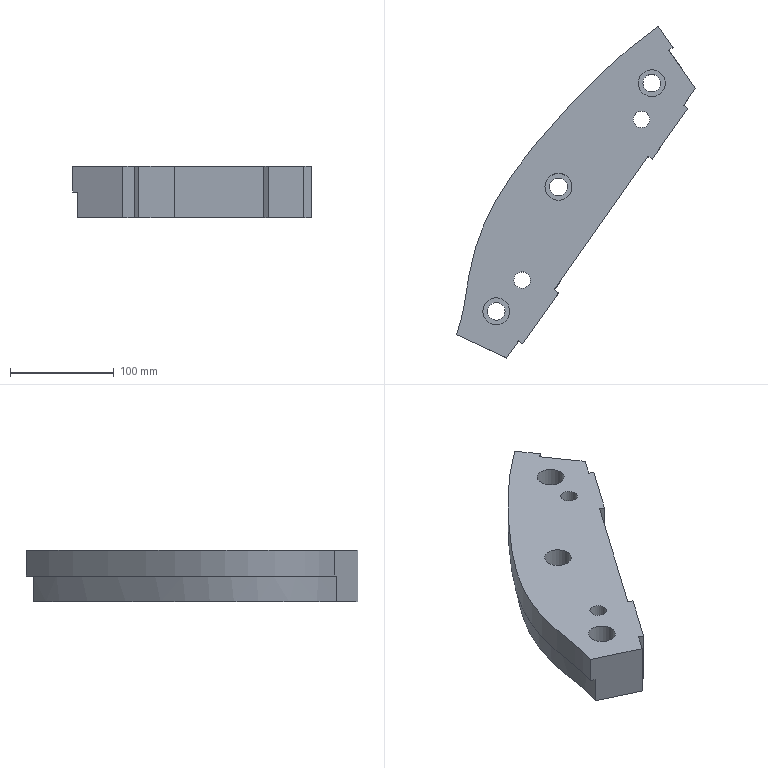Part | NX | features solid 2 | 1 solid | 29 faces | box 230.43 x 320.122 x 50 mm | volume 1328211 mm3 | plane 19 | cylinder 8 | spline 2 | commonest cylinder face diameters 17 x3 26 x3 16 x2
STEP:
#1=CARTESIAN_POINT('',(-554.61,332.835,0.));
#2=VERTEX_POINT('',#1);
#3=CARTESIAN_POINT('',(-554.61,332.835,-50.));
#4=VERTEX_POINT('',#3);
#5=CARTESIAN_POINT('',(-554.61,332.835,-50.));
#6=DIRECTION('',(0.,0.,-1.));
#7=VECTOR('',#6,1000.);
#8=LINE('',#5,#7);
#9=EDGE_CURVE('',#2,#4,#8,.T.);
#10=ORIENTED_EDGE('',*,*,#9,.F.);
#11=CARTESIAN_POINT('',(-566.081,316.452,0.));
#12=VERTEX_POINT('',#11);
#13=CARTESIAN_POINT('',(-736.729,72.741,0.));
#14=DIRECTION('',(0.5736,0.8192,0.));
#15=VECTOR('',#14,1000.);
#16=LINE('',#13,#15);
#17=EDGE_CURVE('',#12,#2,#16,.T.);
#18=ORIENTED_EDGE('',*,*,#17,.F.);
#19=CARTESIAN_POINT('',(-566.081,316.452,-50.));
#20=VERTEX_POINT('',#19);
#21=CARTESIAN_POINT('',(-566.081,316.452,-50.));
#22=DIRECTION('',(0.,0.,1.));
#23=VECTOR('',#22,1000.);
#24=LINE('',#21,#23);
#25=EDGE_CURVE('',#20,#12,#24,.T.);
#26=ORIENTED_EDGE('',*,*,#25,.F.);
#27=CARTESIAN_POINT('',(-736.729,72.741,-50.));
#28=DIRECTION('',(0.5736,0.8192,0.));
#29=VECTOR('',#28,1000.);
#30=LINE('',#27,#29);
#31=EDGE_CURVE('',#20,#4,#30,.T.);
#32=ORIENTED_EDGE('',*,*,#31,.T.);
#33=EDGE_LOOP('',(#10,#18,#26,#32));
#34=FACE_BOUND('',#33,.T.);
#35=CARTESIAN_POINT('',(-736.729,72.741,-50.));
#36=DIRECTION('',(0.8192,-0.5736,0.));
#37=DIRECTION('',(0.5736,0.8192,0.));
#38=AXIS2_PLACEMENT_3D('',#35,#36,#37);
#39=PLANE('',#38);
#40=ADVANCED_FACE('',(#34),#39,.T.);
#41=CARTESIAN_POINT('',(-576.199,372.385,-25.));
#42=VERTEX_POINT('',#41);
#43=CARTESIAN_POINT('',(-576.199,372.385,0.));
#44=VERTEX_POINT('',#43);
#45=CARTESIAN_POINT('',(-576.199,372.385,-50.));
#46=DIRECTION('',(0.,0.,1.));
#47=VECTOR('',#46,1000.);
#48=LINE('',#45,#47);
#49=EDGE_CURVE('',#42,#44,#48,.T.);
#50=ORIENTED_EDGE('',*,*,#49,.F.);
#51=CARTESIAN_POINT('',(-590.538,392.863,-25.));
#52=VERTEX_POINT('',#51);
#53=CARTESIAN_POINT('',(-551.558,337.193,-25.));
#54=DIRECTION('',(0.5736,-0.8192,0.));
#55=VECTOR('',#54,1000.);
#56=LINE('',#53,#55);
#57=EDGE_CURVE('',#52,#42,#56,.T.);
#58=ORIENTED_EDGE('',*,*,#57,.F.);
#59=CARTESIAN_POINT('',(-590.538,392.863,0.));
#60=VERTEX_POINT('',#59);
#61=CARTESIAN_POINT('',(-590.538,392.863,-70.));
#62=DIRECTION('',(0.,0.,1.));
#63=VECTOR('',#62,1000.);
#64=LINE('',#61,#63);
#65=EDGE_CURVE('',#52,#60,#64,.T.);
#66=ORIENTED_EDGE('',*,*,#65,.T.);
#67=CARTESIAN_POINT('',(-551.558,337.193,0.));
#68=DIRECTION('',(-0.5736,0.8192,0.));
#69=VECTOR('',#68,1000.);
#70=LINE('',#67,#69);
#71=EDGE_CURVE('',#44,#60,#70,.T.);
#72=ORIENTED_EDGE('',*,*,#71,.F.);
#73=EDGE_LOOP('',(#50,#58,#66,#72));
#74=FACE_BOUND('',#73,.T.);
#75=CARTESIAN_POINT('',(-551.558,337.193,-50.));
#76=DIRECTION('',(0.8192,0.5736,0.));
#77=DIRECTION('',(-0.5736,0.8192,0.));
#78=AXIS2_PLACEMENT_3D('',#75,#76,#77);
#79=PLANE('',#78);
#80=ADVANCED_FACE('',(#74),#79,.T.);
#81=ORIENTED_EDGE('',*,*,#9,.T.);
#82=CARTESIAN_POINT('',(-591.724,385.839,-50.));
#83=VERTEX_POINT('',#82);
#84=CARTESIAN_POINT('',(-576.978,364.779,-50.));
#85=DIRECTION('',(-0.5736,0.8192,0.));
#86=VECTOR('',#85,1000.);
#87=LINE('',#84,#86);
#88=EDGE_CURVE('',#4,#83,#87,.T.);
#89=ORIENTED_EDGE('',*,*,#88,.T.);
#90=CARTESIAN_POINT('',(-591.724,385.839,-25.));
#91=VERTEX_POINT('',#90);
#92=CARTESIAN_POINT('',(-591.724,385.839,-37.5));
#93=DIRECTION('',(0.,0.,-1.));
#94=VECTOR('',#93,1000.);
#95=LINE('',#92,#94);
#96=EDGE_CURVE('',#91,#83,#95,.T.);
#97=ORIENTED_EDGE('',*,*,#96,.F.);
#98=CARTESIAN_POINT('',(-580.295,369.517,-25.));
#99=VERTEX_POINT('',#98);
#100=CARTESIAN_POINT('',(-555.653,334.325,-25.));
#101=DIRECTION('',(0.5736,-0.8192,0.));
#102=VECTOR('',#101,1000.);
#103=LINE('',#100,#102);
#104=EDGE_CURVE('',#99,#91,#103,.F.);
#105=ORIENTED_EDGE('',*,*,#104,.F.);
#106=CARTESIAN_POINT('',(-580.295,369.517,0.));
#107=VERTEX_POINT('',#106);
#108=CARTESIAN_POINT('',(-580.295,369.517,-50.));
#109=DIRECTION('',(0.,0.,1.));
#110=VECTOR('',#109,1000.);
#111=LINE('',#108,#110);
#112=EDGE_CURVE('',#99,#107,#111,.T.);
#113=ORIENTED_EDGE('',*,*,#112,.T.);
#114=CARTESIAN_POINT('',(-555.653,334.325,0.));
#115=DIRECTION('',(-0.5736,0.8192,0.));
#116=VECTOR('',#115,1000.);
#117=LINE('',#114,#116);
#118=EDGE_CURVE('',#2,#107,#117,.T.);
#119=ORIENTED_EDGE('',*,*,#118,.F.);
#120=EDGE_LOOP('',(#81,#89,#97,#105,#113,#119));
#121=FACE_BOUND('',#120,.T.);
#122=CARTESIAN_POINT('',(-555.653,334.325,-25.));
#123=DIRECTION('',(-0.8192,-0.5736,0.));
#124=DIRECTION('',(0.5736,-0.8192,0.));
#125=AXIS2_PLACEMENT_3D('',#122,#123,#124);
#126=PLANE('',#125);
#127=ADVANCED_FACE('',(#121),#126,.F.);
#128=CARTESIAN_POINT('',(-561.985,313.584,0.));
#129=VERTEX_POINT('',#128);
#130=CARTESIAN_POINT('',(-561.985,313.584,-50.));
#131=VERTEX_POINT('',#130);
#132=CARTESIAN_POINT('',(-561.985,313.584,-50.));
#133=DIRECTION('',(0.,0.,-1.));
#134=VECTOR('',#133,1000.);
#135=LINE('',#132,#134);
#136=EDGE_CURVE('',#129,#131,#135,.T.);
#137=ORIENTED_EDGE('',*,*,#136,.T.);
#138=CARTESIAN_POINT('',(-566.081,316.452,-50.));
#139=DIRECTION('',(0.8192,-0.5736,0.));
#140=VECTOR('',#139,1000.);
#141=LINE('',#138,#140);
#142=EDGE_CURVE('',#20,#131,#141,.T.);
#143=ORIENTED_EDGE('',*,*,#142,.F.);
#144=ORIENTED_EDGE('',*,*,#25,.T.);
#145=CARTESIAN_POINT('',(-566.081,316.452,0.));
#146=DIRECTION('',(0.8192,-0.5736,0.));
#147=VECTOR('',#146,1000.);
#148=LINE('',#145,#147);
#149=EDGE_CURVE('',#12,#129,#148,.T.);
#150=ORIENTED_EDGE('',*,*,#149,.T.);
#151=EDGE_LOOP('',(#137,#143,#144,#150));
#152=FACE_BOUND('',#151,.T.);
#153=CARTESIAN_POINT('',(-566.081,316.452,-50.));
#154=DIRECTION('',(-0.5736,-0.8192,0.));
#155=DIRECTION('',(0.8192,-0.5736,0.));
#156=AXIS2_PLACEMENT_3D('',#153,#154,#155);
#157=PLANE('',#156);
#158=ADVANCED_FACE('',(#152),#157,.F.);
#159=ORIENTED_EDGE('',*,*,#136,.F.);
#160=CARTESIAN_POINT('',(-596.4,264.435,0.));
#161=VERTEX_POINT('',#160);
#162=CARTESIAN_POINT('',(-732.633,69.873,0.));
#163=DIRECTION('',(0.5736,0.8192,0.));
#164=VECTOR('',#163,1000.);
#165=LINE('',#162,#164);
#166=EDGE_CURVE('',#161,#129,#165,.T.);
#167=ORIENTED_EDGE('',*,*,#166,.F.);
#168=CARTESIAN_POINT('',(-596.4,264.435,-50.));
#169=VERTEX_POINT('',#168);
#170=CARTESIAN_POINT('',(-596.4,264.435,-50.));
#171=DIRECTION('',(0.,0.,1.));
#172=VECTOR('',#171,1000.);
#173=LINE('',#170,#172);
#174=EDGE_CURVE('',#169,#161,#173,.T.);
#175=ORIENTED_EDGE('',*,*,#174,.F.);
#176=CARTESIAN_POINT('',(-732.633,69.873,-50.));
#177=DIRECTION('',(0.5736,0.8192,0.));
#178=VECTOR('',#177,1000.);
#179=LINE('',#176,#178);
#180=EDGE_CURVE('',#169,#131,#179,.T.);
#181=ORIENTED_EDGE('',*,*,#180,.T.);
#182=EDGE_LOOP('',(#159,#167,#175,#181));
#183=FACE_BOUND('',#182,.T.);
#184=CARTESIAN_POINT('',(-732.633,69.873,-50.));
#185=DIRECTION('',(0.8192,-0.5736,0.));
#186=DIRECTION('',(0.5736,0.8192,0.));
#187=AXIS2_PLACEMENT_3D('',#184,#185,#186);
#188=PLANE('',#187);
#189=ADVANCED_FACE('',(#183),#188,.T.);
#190=CARTESIAN_POINT('',(-580.295,369.517,-25.));
#191=DIRECTION('',(0.8192,0.5736,0.));
#192=VECTOR('',#191,1000.);
#193=LINE('',#190,#192);
#194=EDGE_CURVE('',#99,#42,#193,.T.);
#195=ORIENTED_EDGE('',*,*,#194,.F.);
#196=ORIENTED_EDGE('',*,*,#104,.T.);
#197=CARTESIAN_POINT('',(-780.467,93.137,-25.));
#198=VERTEX_POINT('',#197);
#199=CARTESIAN_POINT('',(-591.724,385.839,-25.));
#200=CARTESIAN_POINT('',(-603.757,377.032,-25.));
#201=CARTESIAN_POINT('',(-626.864,358.061,-25.));
#202=CARTESIAN_POINT('',(-659.157,326.725,-25.));
#203=CARTESIAN_POINT('',(-689.878,293.729,-25.));
#204=CARTESIAN_POINT('',(-718.933,259.348,-25.));
#205=CARTESIAN_POINT('',(-740.021,228.681,-25.));
#206=CARTESIAN_POINT('',(-753.275,202.223,-25.));
#207=CARTESIAN_POINT('',(-761.052,181.528,-25.));
#208=CARTESIAN_POINT('',(-766.624,160.039,-25.));
#209=CARTESIAN_POINT('',(-769.816,141.694,-25.));
#210=CARTESIAN_POINT('',(-772.179,126.764,-25.));
#211=CARTESIAN_POINT('',(-773.81,117.351,-25.));
#212=CARTESIAN_POINT('',(-775.469,109.707,-25.));
#213=CARTESIAN_POINT('',(-777.049,103.967,-25.));
#214=CARTESIAN_POINT('',(-778.791,98.511,-25.));
#215=CARTESIAN_POINT('',(-779.905,94.938,-25.));
#216=CARTESIAN_POINT('',(-780.467,93.137,-25.));
#217=B_SPLINE_CURVE_WITH_KNOTS('',3,(#199,#200,#201,#202,#203,#204,#205,#206,#207,#208,#209,#210,#211,#212,#213,#214,#215,#216),.UNSPECIFIED.,.F.,.F.,(4,1,1,1,1,1,1,1,1,1,1,1,1,1,1,4),(0.01392,0.1374,0.2609,0.3844,0.5079,0.6314,0.6931,0.7549,0.8166,0.8783,0.9092,0.9401,0.9555,0.971,0.9864,1.002),.UNSPECIFIED.);
#218=EDGE_CURVE('',#91,#198,#217,.T.);
#219=ORIENTED_EDGE('',*,*,#218,.T.);
#220=CARTESIAN_POINT('',(-785.04,95.269,-25.));
#221=VERTEX_POINT('',#220);
#222=CARTESIAN_POINT('',(-785.04,95.269,-25.));
#223=DIRECTION('',(-0.9063,0.4226,0.));
#224=VECTOR('',#223,1000.);
#225=LINE('',#222,#224);
#226=EDGE_CURVE('',#198,#221,#225,.T.);
#227=ORIENTED_EDGE('',*,*,#226,.T.);
#228=CARTESIAN_POINT('',(-590.538,392.863,-25.));
#229=CARTESIAN_POINT('',(-601.77,384.859,-25.));
#230=CARTESIAN_POINT('',(-624.353,366.928,-25.));
#231=CARTESIAN_POINT('',(-656.232,336.831,-25.));
#232=CARTESIAN_POINT('',(-687.219,304.143,-25.));
#233=CARTESIAN_POINT('',(-716.713,270.098,-25.));
#234=CARTESIAN_POINT('',(-738.935,239.768,-25.));
#235=CARTESIAN_POINT('',(-753.526,213.482,-25.));
#236=CARTESIAN_POINT('',(-762.494,192.807,-25.));
#237=CARTESIAN_POINT('',(-769.153,171.263,-25.));
#238=CARTESIAN_POINT('',(-773.765,149.208,-25.));
#239=CARTESIAN_POINT('',(-776.568,130.653,-25.));
#240=CARTESIAN_POINT('',(-778.83,117.715,-25.));
#241=CARTESIAN_POINT('',(-780.455,110.384,-25.));
#242=CARTESIAN_POINT('',(-781.918,105.166,-25.));
#243=CARTESIAN_POINT('',(-783.516,100.148,-25.));
#244=CARTESIAN_POINT('',(-784.526,96.913,-25.));
#245=CARTESIAN_POINT('',(-785.04,95.269,-25.));
#246=B_SPLINE_CURVE_WITH_KNOTS('',3,(#228,#229,#230,#231,#232,#233,#234,#235,#236,#237,#238,#239,#240,#241,#242,#243,#244,#245),.UNSPECIFIED.,.F.,.F.,(4,1,1,1,1,1,1,1,1,1,1,1,1,1,1,4),(0.,0.1128,0.2356,0.3584,0.4812,0.6039,0.6653,0.7267,0.7881,0.8495,0.9109,0.9416,0.9569,0.9723,0.9859,1.),.UNSPECIFIED.);
#247=EDGE_CURVE('',#221,#52,#246,.F.);
#248=ORIENTED_EDGE('',*,*,#247,.T.);
#249=ORIENTED_EDGE('',*,*,#57,.T.);
#250=EDGE_LOOP('',(#195,#196,#219,#227,#248,#249));
#251=FACE_BOUND('',#250,.T.);
#252=CARTESIAN_POINT('',(-782.912,110.608,-25.));
#253=DIRECTION('',(0.,0.,-1.));
#254=DIRECTION('',(-1.,0.,0.));
#255=AXIS2_PLACEMENT_3D('',#252,#253,#254);
#256=PLANE('',#255);
#257=ADVANCED_FACE('',(#251),#256,.T.);
#258=CARTESIAN_POINT('',(-598.729,302.741,-50.));
#259=VERTEX_POINT('',#258);
#260=CARTESIAN_POINT('',(-606.729,302.741,-50.));
#261=DIRECTION('',(0.,0.,1.));
#262=DIRECTION('',(1.,0.,0.));
#263=AXIS2_PLACEMENT_3D('',#260,#261,#262);
#264=CIRCLE('',#263,8.);
#265=EDGE_CURVE('',#259,#259,#264,.T.);
#266=ORIENTED_EDGE('',*,*,#265,.T.);
#267=EDGE_LOOP('',(#266));
#268=FACE_BOUND('',#267,.T.);
#269=CARTESIAN_POINT('',(-713.729,147.741,-50.));
#270=VERTEX_POINT('',#269);
#271=CARTESIAN_POINT('',(-721.729,147.741,-50.));
#272=DIRECTION('',(0.,0.,1.));
#273=DIRECTION('',(1.,0.,0.));
#274=AXIS2_PLACEMENT_3D('',#271,#272,#273);
#275=CIRCLE('',#274,8.);
#276=EDGE_CURVE('',#270,#270,#275,.T.);
#277=ORIENTED_EDGE('',*,*,#276,.T.);
#278=EDGE_LOOP('',(#277));
#279=FACE_BOUND('',#278,.T.);
#280=CARTESIAN_POINT('',(-780.467,93.137,-50.));
#281=VERTEX_POINT('',#280);
#282=CARTESIAN_POINT('',(-780.467,93.137,-50.));
#283=CARTESIAN_POINT('',(-780.262,93.794,-50.));
#284=CARTESIAN_POINT('',(-779.985,94.682,-50.));
#285=CARTESIAN_POINT('',(-779.675,95.672,-50.));
#286=CARTESIAN_POINT('',(-779.473,96.318,-50.));
#287=CARTESIAN_POINT('',(-779.33,96.773,-50.));
#288=CARTESIAN_POINT('',(-779.23,97.095,-50.));
#289=CARTESIAN_POINT('',(-779.177,97.262,-50.));
#290=CARTESIAN_POINT('',(-779.135,97.396,-50.));
#291=CARTESIAN_POINT('',(-779.125,97.427,-50.));
#292=CARTESIAN_POINT('',(-779.066,97.615,-50.));
#293=CARTESIAN_POINT('',(-778.995,97.844,-50.));
#294=CARTESIAN_POINT('',(-778.825,98.383,-50.));
#295=CARTESIAN_POINT('',(-778.479,99.488,-50.));
#296=CARTESIAN_POINT('',(-778.019,100.956,-50.));
#297=CARTESIAN_POINT('',(-777.588,102.341,-50.));
#298=CARTESIAN_POINT('',(-777.324,103.195,-50.));
#299=CARTESIAN_POINT('',(-777.198,103.607,-50.));
#300=CARTESIAN_POINT('',(-777.131,103.831,-50.));
#301=CARTESIAN_POINT('',(-777.117,103.876,-50.));
#302=CARTESIAN_POINT('',(-776.998,104.278,-50.));
#303=CARTESIAN_POINT('',(-776.877,104.691,-50.));
#304=CARTESIAN_POINT('',(-776.651,105.476,-50.));
#305=CARTESIAN_POINT('',(-776.344,106.576,-50.));
#306=CARTESIAN_POINT('',(-775.984,107.923,-50.));
#307=CARTESIAN_POINT('',(-775.521,109.737,-50.));
#308=CARTESIAN_POINT('',(-775.082,111.576,-50.));
#309=CARTESIAN_POINT('',(-774.716,113.227,-50.));
#310=CARTESIAN_POINT('',(-774.517,114.154,-50.));
#311=CARTESIAN_POINT('',(-774.358,114.921,-50.));
#312=CARTESIAN_POINT('',(-774.254,115.432,-50.));
#313=CARTESIAN_POINT('',(-774.093,116.231,-50.));
#314=CARTESIAN_POINT('',(-773.816,117.643,-50.));
#315=CARTESIAN_POINT('',(-773.484,119.411,-50.));
#316=CARTESIAN_POINT('',(-773.143,121.304,-50.));
#317=CARTESIAN_POINT('',(-772.924,122.545,-50.));
#318=CARTESIAN_POINT('',(-772.746,123.57,-50.));
#319=CARTESIAN_POINT('',(-772.611,124.357,-50.));
#320=CARTESIAN_POINT('',(-772.499,125.02,-50.));
#321=CARTESIAN_POINT('',(-772.417,125.507,-50.));
#322=CARTESIAN_POINT('',(-772.374,125.761,-50.));
#323=CARTESIAN_POINT('',(-772.33,126.027,-50.));
#324=CARTESIAN_POINT('',(-772.332,126.013,-50.));
#325=CARTESIAN_POINT('',(-772.318,126.1,-50.));
#326=CARTESIAN_POINT('',(-772.298,126.219,-50.));
#327=CARTESIAN_POINT('',(-772.259,126.454,-50.));
#328=CARTESIAN_POINT('',(-772.204,126.791,-50.));
#329=CARTESIAN_POINT('',(-772.115,127.33,-50.));
#330=CARTESIAN_POINT('',(-771.979,128.166,-50.));
#331=CARTESIAN_POINT('',(-771.773,129.43,-50.));
#332=CARTESIAN_POINT('',(-771.525,130.954,-50.));
#333=CARTESIAN_POINT('',(-771.235,132.74,-50.));
#334=CARTESIAN_POINT('',(-770.959,134.436,-50.));
#335=CARTESIAN_POINT('',(-770.745,135.757,-50.));
#336=CARTESIAN_POINT('',(-770.622,136.513,-50.));
#337=CARTESIAN_POINT('',(-770.514,137.183,-50.));
#338=CARTESIAN_POINT('',(-770.456,137.54,-50.));
#339=CARTESIAN_POINT('',(-770.362,138.117,-50.));
#340=CARTESIAN_POINT('',(-770.208,139.059,-50.));
#341=CARTESIAN_POINT('',(-769.99,140.385,-50.));
#342=CARTESIAN_POINT('',(-769.741,141.888,-50.));
#343=CARTESIAN_POINT('',(-769.42,143.795,-50.));
#344=CARTESIAN_POINT('',(-769.118,145.556,-50.));
#345=CARTESIAN_POINT('',(-768.875,146.945,-50.));
#346=CARTESIAN_POINT('',(-768.736,147.73,-50.));
#347=CARTESIAN_POINT('',(-768.649,148.216,-50.));
#348=CARTESIAN_POINT('',(-768.506,149.007,-50.));
#349=CARTESIAN_POINT('',(-768.334,149.947,-50.));
#350=CARTESIAN_POINT('',(-768.022,151.628,-50.));
#351=CARTESIAN_POINT('',(-767.576,153.95,-50.));
#352=CARTESIAN_POINT('',(-767.021,156.711,-50.));
#353=CARTESIAN_POINT('',(-766.486,159.267,-50.));
#354=CARTESIAN_POINT('',(-765.833,162.239,-50.));
#355=CARTESIAN_POINT('',(-764.964,165.986,-50.));
#356=CARTESIAN_POINT('',(-763.812,170.613,-50.));
#357=CARTESIAN_POINT('',(-762.331,176.008,-50.));
#358=CARTESIAN_POINT('',(-760.797,181.117,-50.));
#359=CARTESIAN_POINT('',(-759.02,186.518,-50.));
#360=CARTESIAN_POINT('',(-757.127,191.776,-50.));
#361=CARTESIAN_POINT('',(-755.092,196.987,-50.));
#362=CARTESIAN_POINT('',(-752.888,202.202,-50.));
#363=CARTESIAN_POINT('',(-750.656,207.118,-50.));
#364=CARTESIAN_POINT('',(-748.243,212.109,-50.));
#365=CARTESIAN_POINT('',(-746.108,216.259,-50.));
#366=CARTESIAN_POINT('',(-744.336,219.558,-50.));
#367=CARTESIAN_POINT('',(-742.933,222.096,-50.));
#368=CARTESIAN_POINT('',(-741.633,224.387,-50.));
#369=CARTESIAN_POINT('',(-739.798,227.541,-50.));
#370=CARTESIAN_POINT('',(-737.429,231.467,-50.));
#371=CARTESIAN_POINT('',(-734.915,235.446,-50.));
#372=CARTESIAN_POINT('',(-732.852,238.607,-50.));
#373=CARTESIAN_POINT('',(-731.201,241.082,-50.));
#374=CARTESIAN_POINT('',(-729.76,243.199,-50.));
#375=CARTESIAN_POINT('',(-727.695,246.184,-50.));
#376=CARTESIAN_POINT('',(-725.035,249.928,-50.));
#377=CARTESIAN_POINT('',(-722.23,253.752,-50.));
#378=CARTESIAN_POINT('',(-720.181,256.484,-50.));
#379=CARTESIAN_POINT('',(-719.01,258.027,-50.));
#380=CARTESIAN_POINT('',(-718.06,259.271,-50.));
#381=CARTESIAN_POINT('',(-717.336,260.211,-50.));
#382=CARTESIAN_POINT('',(-716.279,261.579,-50.));
#383=CARTESIAN_POINT('',(-714.439,263.939,-50.));
#384=CARTESIAN_POINT('',(-711.711,267.383,-50.));
#385=CARTESIAN_POINT('',(-708.319,271.579,-50.));
#386=CARTESIAN_POINT('',(-703.622,277.279,-50.));
#387=CARTESIAN_POINT('',(-698.678,283.119,-50.));
#388=CARTESIAN_POINT('',(-694.112,288.379,-50.));
#389=CARTESIAN_POINT('',(-691.465,291.394,-50.));
#390=CARTESIAN_POINT('',(-689.376,293.754,-50.));
#391=CARTESIAN_POINT('',(-687.528,295.827,-50.));
#392=CARTESIAN_POINT('',(-684.978,298.673,-50.));
#393=CARTESIAN_POINT('',(-680.548,303.571,-50.));
#394=CARTESIAN_POINT('',(-675.452,309.104,-50.));
#395=CARTESIAN_POINT('',(-670.35,314.544,-50.));
#396=CARTESIAN_POINT('',(-666.511,318.586,-50.));
#397=CARTESIAN_POINT('',(-663.32,321.904,-50.));
#398=CARTESIAN_POINT('',(-660.732,324.57,-50.));
#399=CARTESIAN_POINT('',(-658.874,326.471,-50.));
#400=CARTESIAN_POINT('',(-656.69,328.693,-50.));
#401=CARTESIAN_POINT('',(-653.912,331.497,-50.));
#402=CARTESIAN_POINT('',(-649.037,336.363,-50.));
#403=CARTESIAN_POINT('',(-643.589,341.679,-50.));
#404=CARTESIAN_POINT('',(-638.229,346.782,-50.));
#405=CARTESIAN_POINT('',(-634.262,350.495,-50.));
#406=CARTESIAN_POINT('',(-630.989,353.503,-50.));
#407=CARTESIAN_POINT('',(-628.733,355.548,-50.));
#408=CARTESIAN_POINT('',(-627.429,356.722,-50.));
#409=CARTESIAN_POINT('',(-626.514,357.542,-50.));
#410=CARTESIAN_POINT('',(-625.373,358.559,-50.));
#411=CARTESIAN_POINT('',(-623.932,359.836,-50.));
#412=CARTESIAN_POINT('',(-621.374,362.083,-50.));
#413=CARTESIAN_POINT('',(-617.744,365.218,-50.));
#414=CARTESIAN_POINT('',(-613.387,368.893,-50.));
#415=CARTESIAN_POINT('',(-607.59,373.666,-50.));
#416=CARTESIAN_POINT('',(-600.362,379.399,-50.));
#417=CARTESIAN_POINT('',(-594.6,383.734,-50.));
#418=CARTESIAN_POINT('',(-591.724,385.839,-50.));
#419=B_SPLINE_CURVE_WITH_KNOTS('',3,(#282,#283,#284,#285,#286,#287,#288,#289,#290,#291,#292,#293,#294,#295,#296,#297,#298,#299,#300,#301,#302,#303,#304,#305,#306,#307,#308,#309,#310,#311,#312,#313,#314,#315,#316,#317,#318,#319,#320,#321,#322,#323,#324,#325,#326,#327,#328,#329,#330,#331,#332,#333,#334,#335,#336,#337,#338,#339,#340,#341,#342,#343,#344,#345,#346,#347,#348,#349,#350,#351,#352,#353,#354,#355,#356,#357,#358,#359,#360,#361,#362,#363,#364,#365,#366,#367,#368,#369,#370,#371,#372,#373,#374,#375,#376,#377,#378,#379,#380,#381,#382,#383,#384,#385,#386,#387,#388,#389,#390,#391,#392,#393,#394,#395,#396,#397,#398,#399,#400,#401,#402,#403,#404,#405,#406,#407,#408,#409,#410,#411,#412,#413,#414,#415,#416,#417,#418),.UNSPECIFIED.,.F.,.F.,(4,1,1,1,1,1,1,1,1,1,1,1,1,1,1,1,1,1,1,1,1,1,1,1,1,1,1,1,1,1,1,1,1,1,1,1,1,1,1,1,1,1,1,1,1,1,1,1,1,1,1,1,1,1,1,1,1,1,1,1,1,1,1,1,1,1,1,1,1,1,1,1,1,1,1,1,1,1,1,1,1,1,1,1,1,1,1,1,1,1,1,1,1,1,1,1,1,1,1,1,1,1,1,1,1,1,1,1,1,1,1,1,1,1,1,1,1,1,1,1,1,1,1,1,1,1,1,1,1,1,1,1,1,1,4),(0.,0.003906,0.005859,0.007812,0.009766,0.01074,0.01172,0.01221,0.01245,0.0127,0.01318,0.01367,0.01562,0.01953,0.02344,0.02734,0.0293,0.03027,0.03125,0.03223,0.0332,0.03516,0.03906,0.04297,0.04688,0.05469,0.05859,0.06055,0.0625,0.06445,0.06641,0.07031,0.07812,0.08203,0.08594,0.08789,0.08984,0.0918,0.09277,0.09326,0.09375,0.09424,0.09473,0.0957,0.09766,0.09961,0.1016,0.1055,0.1094,0.1133,0.1172,0.1211,0.123,0.124,0.125,0.126,0.127,0.1289,0.1328,0.1367,0.1406,0.1484,0.1523,0.1543,0.1562,0.1582,0.1602,0.1641,0.1719,0.1797,0.1875,0.1953,0.2031,0.2188,0.2344,0.25,0.2656,0.2812,0.2969,0.3125,0.3281,0.3438,0.3594,0.3672,0.375,0.3828,0.3906,0.4062,0.4219,0.4297,0.4375,0.4453,0.4531,0.4688,0.4844,0.4922,0.4961,0.5,0.5039,0.5078,0.5156,0.5312,0.5469,0.5625,0.5938,0.6094,0.6172,0.625,0.6328,0.6406,0.6562,0.6875,0.7031,0.7188,0.7344,0.7422,0.75,0.7578,0.7656,0.7812,0.8125,0.8281,0.8438,0.8594,0.8672,0.8711,0.875,0.8789,0.8828,0.8906,0.9062,0.9219,0.9375,0.9688,1.),.UNSPECIFIED.);
#420=EDGE_CURVE('',#83,#281,#419,.F.);
#421=ORIENTED_EDGE('',*,*,#420,.F.);
#422=ORIENTED_EDGE('',*,*,#88,.F.);
#423=ORIENTED_EDGE('',*,*,#31,.F.);
#424=ORIENTED_EDGE('',*,*,#142,.T.);
#425=ORIENTED_EDGE('',*,*,#180,.F.);
#426=CARTESIAN_POINT('',(-600.496,267.302,-50.));
#427=VERTEX_POINT('',#426);
#428=CARTESIAN_POINT('',(-600.496,267.302,-50.));
#429=DIRECTION('',(0.8192,-0.5736,0.));
#430=VECTOR('',#429,1000.);
#431=LINE('',#428,#430);
#432=EDGE_CURVE('',#427,#169,#431,.T.);
#433=ORIENTED_EDGE('',*,*,#432,.F.);
#434=CARTESIAN_POINT('',(-690.843,138.273,-50.));
#435=VERTEX_POINT('',#434);
#436=CARTESIAN_POINT('',(-736.729,72.741,-50.));
#437=DIRECTION('',(0.5736,0.8192,0.));
#438=VECTOR('',#437,1000.);
#439=LINE('',#436,#438);
#440=EDGE_CURVE('',#435,#427,#439,.T.);
#441=ORIENTED_EDGE('',*,*,#440,.F.);
#442=CARTESIAN_POINT('',(-686.747,135.406,-50.));
#443=VERTEX_POINT('',#442);
#444=CARTESIAN_POINT('',(-690.843,138.273,-50.));
#445=DIRECTION('',(0.8192,-0.5736,0.));
#446=VECTOR('',#445,1000.);
#447=LINE('',#444,#446);
#448=EDGE_CURVE('',#435,#443,#447,.T.);
#449=ORIENTED_EDGE('',*,*,#448,.T.);
#450=CARTESIAN_POINT('',(-721.162,86.256,-50.));
#451=VERTEX_POINT('',#450);
#452=CARTESIAN_POINT('',(-874.602,-132.879,-50.));
#453=DIRECTION('',(0.5736,0.8192,0.));
#454=VECTOR('',#453,1000.);
#455=LINE('',#452,#454);
#456=EDGE_CURVE('',#451,#443,#455,.T.);
#457=ORIENTED_EDGE('',*,*,#456,.F.);
#458=CARTESIAN_POINT('',(-725.257,89.124,-50.));
#459=VERTEX_POINT('',#458);
#460=CARTESIAN_POINT('',(-725.257,89.124,-50.));
#461=DIRECTION('',(0.8192,-0.5736,0.));
#462=VECTOR('',#461,1000.);
#463=LINE('',#460,#462);
#464=EDGE_CURVE('',#459,#451,#463,.T.);
#465=ORIENTED_EDGE('',*,*,#464,.F.);
#466=CARTESIAN_POINT('',(-736.729,72.741,-50.));
#467=VERTEX_POINT('',#466);
#468=CARTESIAN_POINT('',(-736.729,72.741,-50.));
#469=DIRECTION('',(0.5736,0.8192,0.));
#470=VECTOR('',#469,1000.);
#471=LINE('',#468,#470);
#472=EDGE_CURVE('',#467,#459,#471,.T.);
#473=ORIENTED_EDGE('',*,*,#472,.F.);
#474=CARTESIAN_POINT('',(-785.04,95.269,-50.));
#475=DIRECTION('',(0.9063,-0.4226,0.));
#476=VECTOR('',#475,1000.);
#477=LINE('',#474,#476);
#478=EDGE_CURVE('',#281,#467,#477,.T.);
#479=ORIENTED_EDGE('',*,*,#478,.F.);
#480=EDGE_LOOP('',(#421,#422,#423,#424,#425,#433,#441,#449,#457,#465,#473,#479));
#481=FACE_BOUND('',#480,.T.);
#482=CARTESIAN_POINT('',(-695.229,237.741,-50.));
#483=VERTEX_POINT('',#482);
#484=CARTESIAN_POINT('',(-686.729,237.741,-50.));
#485=DIRECTION('',(0.,0.,-1.));
#486=DIRECTION('',(-1.,0.,0.));
#487=AXIS2_PLACEMENT_3D('',#484,#485,#486);
#488=CIRCLE('',#487,8.5);
#489=EDGE_CURVE('',#483,#483,#488,.T.);
#490=ORIENTED_EDGE('',*,*,#489,.F.);
#491=EDGE_LOOP('',(#490));
#492=FACE_BOUND('',#491,.T.);
#493=CARTESIAN_POINT('',(-605.229,337.741,-50.));
#494=VERTEX_POINT('',#493);
#495=CARTESIAN_POINT('',(-596.729,337.741,-50.));
#496=DIRECTION('',(0.,0.,-1.));
#497=DIRECTION('',(-1.,0.,0.));
#498=AXIS2_PLACEMENT_3D('',#495,#496,#497);
#499=CIRCLE('',#498,8.5);
#500=EDGE_CURVE('',#494,#494,#499,.T.);
#501=ORIENTED_EDGE('',*,*,#500,.F.);
#502=EDGE_LOOP('',(#501));
#503=FACE_BOUND('',#502,.T.);
#504=CARTESIAN_POINT('',(-755.229,117.741,-50.));
#505=VERTEX_POINT('',#504);
#506=CARTESIAN_POINT('',(-746.729,117.741,-50.));
#507=DIRECTION('',(0.,0.,-1.));
#508=DIRECTION('',(-1.,0.,0.));
#509=AXIS2_PLACEMENT_3D('',#506,#507,#508);
#510=CIRCLE('',#509,8.5);
#511=EDGE_CURVE('',#505,#505,#510,.T.);
#512=ORIENTED_EDGE('',*,*,#511,.F.);
#513=EDGE_LOOP('',(#512));
#514=FACE_BOUND('',#513,.T.);
#515=CARTESIAN_POINT('',(-877.439,-108.839,-50.));
#516=DIRECTION('',(0.,0.,1.));
#517=DIRECTION('',(1.,0.,0.));
#518=AXIS2_PLACEMENT_3D('',#515,#516,#517);
#519=PLANE('',#518);
#520=ADVANCED_FACE('',(#268,#279,#481,#492,#503,#514),#519,.F.);
#521=CARTESIAN_POINT('',(-598.729,302.741,0.));
#522=VERTEX_POINT('',#521);
#523=CARTESIAN_POINT('',(-606.729,302.741,0.));
#524=DIRECTION('',(0.,0.,1.));
#525=DIRECTION('',(1.,0.,0.));
#526=AXIS2_PLACEMENT_3D('',#523,#524,#525);
#527=CIRCLE('',#526,8.);
#528=EDGE_CURVE('',#522,#522,#527,.F.);
#529=ORIENTED_EDGE('',*,*,#528,.T.);
#530=EDGE_LOOP('',(#529));
#531=FACE_BOUND('',#530,.T.);
#532=CARTESIAN_POINT('',(-713.729,147.741,0.));
#533=VERTEX_POINT('',#532);
#534=CARTESIAN_POINT('',(-721.729,147.741,0.));
#535=DIRECTION('',(0.,0.,1.));
#536=DIRECTION('',(1.,0.,0.));
#537=AXIS2_PLACEMENT_3D('',#534,#535,#536);
#538=CIRCLE('',#537,8.);
#539=EDGE_CURVE('',#533,#533,#538,.F.);
#540=ORIENTED_EDGE('',*,*,#539,.T.);
#541=EDGE_LOOP('',(#540));
#542=FACE_BOUND('',#541,.T.);
#543=ORIENTED_EDGE('',*,*,#118,.T.);
#544=CARTESIAN_POINT('',(-580.295,369.517,0.));
#545=DIRECTION('',(0.8192,0.5736,0.));
#546=VECTOR('',#545,1000.);
#547=LINE('',#544,#546);
#548=EDGE_CURVE('',#107,#44,#547,.T.);
#549=ORIENTED_EDGE('',*,*,#548,.T.);
#550=ORIENTED_EDGE('',*,*,#71,.T.);
#551=CARTESIAN_POINT('',(-785.04,95.269,0.));
#552=VERTEX_POINT('',#551);
#553=CARTESIAN_POINT('',(-590.538,392.863,0.));
#554=CARTESIAN_POINT('',(-601.77,384.859,0.));
#555=CARTESIAN_POINT('',(-624.353,366.928,0.));
#556=CARTESIAN_POINT('',(-656.232,336.831,0.));
#557=CARTESIAN_POINT('',(-687.219,304.143,0.));
#558=CARTESIAN_POINT('',(-716.713,270.098,0.));
#559=CARTESIAN_POINT('',(-738.935,239.768,0.));
#560=CARTESIAN_POINT('',(-753.526,213.482,0.));
#561=CARTESIAN_POINT('',(-762.494,192.807,0.));
#562=CARTESIAN_POINT('',(-769.153,171.263,0.));
#563=CARTESIAN_POINT('',(-773.765,149.208,0.));
#564=CARTESIAN_POINT('',(-776.568,130.653,0.));
#565=CARTESIAN_POINT('',(-778.83,117.715,0.));
#566=CARTESIAN_POINT('',(-780.455,110.384,0.));
#567=CARTESIAN_POINT('',(-781.918,105.166,0.));
#568=CARTESIAN_POINT('',(-783.516,100.148,0.));
#569=CARTESIAN_POINT('',(-784.526,96.913,0.));
#570=CARTESIAN_POINT('',(-785.04,95.269,0.));
#571=B_SPLINE_CURVE_WITH_KNOTS('',3,(#553,#554,#555,#556,#557,#558,#559,#560,#561,#562,#563,#564,#565,#566,#567,#568,#569,#570),.UNSPECIFIED.,.F.,.F.,(4,1,1,1,1,1,1,1,1,1,1,1,1,1,1,4),(0.,0.1128,0.2356,0.3584,0.4812,0.6039,0.6653,0.7267,0.7881,0.8495,0.9109,0.9416,0.9569,0.9723,0.9859,1.),.UNSPECIFIED.);
#572=EDGE_CURVE('',#60,#552,#571,.T.);
#573=ORIENTED_EDGE('',*,*,#572,.T.);
#574=CARTESIAN_POINT('',(-736.729,72.741,0.));
#575=VERTEX_POINT('',#574);
#576=CARTESIAN_POINT('',(-785.04,95.269,0.));
#577=DIRECTION('',(0.9063,-0.4226,0.));
#578=VECTOR('',#577,1000.);
#579=LINE('',#576,#578);
#580=EDGE_CURVE('',#552,#575,#579,.T.);
#581=ORIENTED_EDGE('',*,*,#580,.T.);
#582=CARTESIAN_POINT('',(-725.257,89.124,0.));
#583=VERTEX_POINT('',#582);
#584=CARTESIAN_POINT('',(-736.729,72.741,0.));
#585=DIRECTION('',(0.5736,0.8192,0.));
#586=VECTOR('',#585,1000.);
#587=LINE('',#584,#586);
#588=EDGE_CURVE('',#575,#583,#587,.T.);
#589=ORIENTED_EDGE('',*,*,#588,.T.);
#590=CARTESIAN_POINT('',(-721.162,86.256,0.));
#591=VERTEX_POINT('',#590);
#592=CARTESIAN_POINT('',(-725.257,89.124,0.));
#593=DIRECTION('',(0.8192,-0.5736,0.));
#594=VECTOR('',#593,1000.);
#595=LINE('',#592,#594);
#596=EDGE_CURVE('',#583,#591,#595,.T.);
#597=ORIENTED_EDGE('',*,*,#596,.T.);
#598=CARTESIAN_POINT('',(-686.747,135.406,0.));
#599=VERTEX_POINT('',#598);
#600=CARTESIAN_POINT('',(-874.602,-132.879,0.));
#601=DIRECTION('',(0.5736,0.8192,0.));
#602=VECTOR('',#601,1000.);
#603=LINE('',#600,#602);
#604=EDGE_CURVE('',#591,#599,#603,.T.);
#605=ORIENTED_EDGE('',*,*,#604,.T.);
#606=CARTESIAN_POINT('',(-690.843,138.273,0.));
#607=VERTEX_POINT('',#606);
#608=CARTESIAN_POINT('',(-690.843,138.273,0.));
#609=DIRECTION('',(0.8192,-0.5736,0.));
#610=VECTOR('',#609,1000.);
#611=LINE('',#608,#610);
#612=EDGE_CURVE('',#607,#599,#611,.T.);
#613=ORIENTED_EDGE('',*,*,#612,.F.);
#614=CARTESIAN_POINT('',(-600.496,267.302,0.));
#615=VERTEX_POINT('',#614);
#616=CARTESIAN_POINT('',(-736.729,72.741,0.));
#617=DIRECTION('',(0.5736,0.8192,0.));
#618=VECTOR('',#617,1000.);
#619=LINE('',#616,#618);
#620=EDGE_CURVE('',#607,#615,#619,.T.);
#621=ORIENTED_EDGE('',*,*,#620,.T.);
#622=CARTESIAN_POINT('',(-600.496,267.302,0.));
#623=DIRECTION('',(0.8192,-0.5736,0.));
#624=VECTOR('',#623,1000.);
#625=LINE('',#622,#624);
#626=EDGE_CURVE('',#615,#161,#625,.T.);
#627=ORIENTED_EDGE('',*,*,#626,.T.);
#628=ORIENTED_EDGE('',*,*,#166,.T.);
#629=ORIENTED_EDGE('',*,*,#149,.F.);
#630=ORIENTED_EDGE('',*,*,#17,.T.);
#631=EDGE_LOOP('',(#543,#549,#550,#573,#581,#589,#597,#605,#613,#621,#627,#628,#629,#630));
#632=FACE_BOUND('',#631,.T.);
#633=CARTESIAN_POINT('',(-699.729,237.741,0.));
#634=VERTEX_POINT('',#633);
#635=CARTESIAN_POINT('',(-686.729,237.741,0.));
#636=DIRECTION('',(0.,0.,-1.));
#637=DIRECTION('',(-1.,0.,0.));
#638=AXIS2_PLACEMENT_3D('',#635,#636,#637);
#639=CIRCLE('',#638,13.);
#640=EDGE_CURVE('',#634,#634,#639,.T.);
#641=ORIENTED_EDGE('',*,*,#640,.T.);
#642=EDGE_LOOP('',(#641));
#643=FACE_BOUND('',#642,.T.);
#644=CARTESIAN_POINT('',(-609.729,337.741,0.));
#645=VERTEX_POINT('',#644);
#646=CARTESIAN_POINT('',(-596.729,337.741,0.));
#647=DIRECTION('',(0.,0.,-1.));
#648=DIRECTION('',(-1.,0.,0.));
#649=AXIS2_PLACEMENT_3D('',#646,#647,#648);
#650=CIRCLE('',#649,13.);
#651=EDGE_CURVE('',#645,#645,#650,.T.);
#652=ORIENTED_EDGE('',*,*,#651,.T.);
#653=EDGE_LOOP('',(#652));
#654=FACE_BOUND('',#653,.T.);
#655=CARTESIAN_POINT('',(-759.729,117.741,0.));
#656=VERTEX_POINT('',#655);
#657=CARTESIAN_POINT('',(-746.729,117.741,0.));
#658=DIRECTION('',(0.,0.,-1.));
#659=DIRECTION('',(-1.,0.,0.));
#660=AXIS2_PLACEMENT_3D('',#657,#658,#659);
#661=CIRCLE('',#660,13.);
#662=EDGE_CURVE('',#656,#656,#661,.T.);
#663=ORIENTED_EDGE('',*,*,#662,.T.);
#664=EDGE_LOOP('',(#663));
#665=FACE_BOUND('',#664,.T.);
#666=CARTESIAN_POINT('',(-687.45,66.093,0.));
#667=DIRECTION('',(0.,0.,1.));
#668=DIRECTION('',(0.5736,0.8192,0.));
#669=AXIS2_PLACEMENT_3D('',#666,#667,#668);
#670=PLANE('',#669);
#671=ADVANCED_FACE('',(#531,#542,#632,#643,#654,#665),#670,.T.);
#672=CARTESIAN_POINT('',(-733.729,117.741,-25.));
#673=VERTEX_POINT('',#672);
#674=CARTESIAN_POINT('',(-746.729,117.741,-25.));
#675=DIRECTION('',(0.,0.,1.));
#676=DIRECTION('',(1.,0.,0.));
#677=AXIS2_PLACEMENT_3D('',#674,#675,#676);
#678=CIRCLE('',#677,13.);
#679=EDGE_CURVE('',#673,#673,#678,.T.);
#680=ORIENTED_EDGE('',*,*,#679,.T.);
#681=EDGE_LOOP('',(#680));
#682=FACE_BOUND('',#681,.T.);
#683=CARTESIAN_POINT('',(-755.229,117.741,-25.));
#684=VERTEX_POINT('',#683);
#685=CARTESIAN_POINT('',(-746.729,117.741,-25.));
#686=DIRECTION('',(0.,0.,-1.));
#687=DIRECTION('',(-1.,0.,0.));
#688=AXIS2_PLACEMENT_3D('',#685,#686,#687);
#689=CIRCLE('',#688,8.5);
#690=EDGE_CURVE('',#684,#684,#689,.F.);
#691=ORIENTED_EDGE('',*,*,#690,.F.);
#692=EDGE_LOOP('',(#691));
#693=FACE_BOUND('',#692,.T.);
#694=CARTESIAN_POINT('',(-746.729,117.741,-25.));
#695=DIRECTION('',(0.,0.,-1.));
#696=DIRECTION('',(-1.,0.,0.));
#697=AXIS2_PLACEMENT_3D('',#694,#695,#696);
#698=PLANE('',#697);
#699=ADVANCED_FACE('',(#682,#693),#698,.F.);
#700=ORIENTED_EDGE('',*,*,#511,.T.);
#701=EDGE_LOOP('',(#700));
#702=FACE_BOUND('',#701,.T.);
#703=ORIENTED_EDGE('',*,*,#690,.T.);
#704=EDGE_LOOP('',(#703));
#705=FACE_BOUND('',#704,.T.);
#706=CARTESIAN_POINT('',(-746.729,117.741,-75.));
#707=DIRECTION('',(0.,0.,1.));
#708=DIRECTION('',(1.,0.,0.));
#709=AXIS2_PLACEMENT_3D('',#706,#707,#708);
#710=CYLINDRICAL_SURFACE('',#709,8.5);
#711=ADVANCED_FACE('',(#702,#705),#710,.F.);
#712=ORIENTED_EDGE('',*,*,#662,.F.);
#713=EDGE_LOOP('',(#712));
#714=FACE_BOUND('',#713,.T.);
#715=ORIENTED_EDGE('',*,*,#679,.F.);
#716=EDGE_LOOP('',(#715));
#717=FACE_BOUND('',#716,.T.);
#718=CARTESIAN_POINT('',(-746.729,117.741,-25.));
#719=DIRECTION('',(0.,0.,1.));
#720=DIRECTION('',(1.,0.,0.));
#721=AXIS2_PLACEMENT_3D('',#718,#719,#720);
#722=CYLINDRICAL_SURFACE('',#721,13.);
#723=ADVANCED_FACE('',(#714,#717),#722,.F.);
#724=CARTESIAN_POINT('',(-673.729,237.741,-25.));
#725=VERTEX_POINT('',#724);
#726=CARTESIAN_POINT('',(-686.729,237.741,-25.));
#727=DIRECTION('',(0.,0.,1.));
#728=DIRECTION('',(1.,0.,0.));
#729=AXIS2_PLACEMENT_3D('',#726,#727,#728);
#730=CIRCLE('',#729,13.);
#731=EDGE_CURVE('',#725,#725,#730,.T.);
#732=ORIENTED_EDGE('',*,*,#731,.T.);
#733=EDGE_LOOP('',(#732));
#734=FACE_BOUND('',#733,.T.);
#735=CARTESIAN_POINT('',(-695.229,237.741,-25.));
#736=VERTEX_POINT('',#735);
#737=CARTESIAN_POINT('',(-686.729,237.741,-25.));
#738=DIRECTION('',(0.,0.,-1.));
#739=DIRECTION('',(-1.,0.,0.));
#740=AXIS2_PLACEMENT_3D('',#737,#738,#739);
#741=CIRCLE('',#740,8.5);
#742=EDGE_CURVE('',#736,#736,#741,.F.);
#743=ORIENTED_EDGE('',*,*,#742,.F.);
#744=EDGE_LOOP('',(#743));
#745=FACE_BOUND('',#744,.T.);
#746=CARTESIAN_POINT('',(-686.729,237.741,-25.));
#747=DIRECTION('',(0.,0.,-1.));
#748=DIRECTION('',(-1.,0.,0.));
#749=AXIS2_PLACEMENT_3D('',#746,#747,#748);
#750=PLANE('',#749);
#751=ADVANCED_FACE('',(#734,#745),#750,.F.);
#752=ORIENTED_EDGE('',*,*,#640,.F.);
#753=EDGE_LOOP('',(#752));
#754=FACE_BOUND('',#753,.T.);
#755=ORIENTED_EDGE('',*,*,#731,.F.);
#756=EDGE_LOOP('',(#755));
#757=FACE_BOUND('',#756,.T.);
#758=CARTESIAN_POINT('',(-686.729,237.741,-25.));
#759=DIRECTION('',(0.,0.,1.));
#760=DIRECTION('',(1.,0.,0.));
#761=AXIS2_PLACEMENT_3D('',#758,#759,#760);
#762=CYLINDRICAL_SURFACE('',#761,13.);
#763=ADVANCED_FACE('',(#754,#757),#762,.F.);
#764=ORIENTED_EDGE('',*,*,#489,.T.);
#765=EDGE_LOOP('',(#764));
#766=FACE_BOUND('',#765,.T.);
#767=ORIENTED_EDGE('',*,*,#742,.T.);
#768=EDGE_LOOP('',(#767));
#769=FACE_BOUND('',#768,.T.);
#770=CARTESIAN_POINT('',(-686.729,237.741,-75.));
#771=DIRECTION('',(0.,0.,1.));
#772=DIRECTION('',(1.,0.,0.));
#773=AXIS2_PLACEMENT_3D('',#770,#771,#772);
#774=CYLINDRICAL_SURFACE('',#773,8.5);
#775=ADVANCED_FACE('',(#766,#769),#774,.F.);
#776=CARTESIAN_POINT('',(-605.229,337.741,-25.));
#777=VERTEX_POINT('',#776);
#778=CARTESIAN_POINT('',(-596.729,337.741,-25.));
#779=DIRECTION('',(0.,0.,-1.));
#780=DIRECTION('',(-1.,0.,0.));
#781=AXIS2_PLACEMENT_3D('',#778,#779,#780);
#782=CIRCLE('',#781,8.5);
#783=EDGE_CURVE('',#777,#777,#782,.F.);
#784=ORIENTED_EDGE('',*,*,#783,.F.);
#785=EDGE_LOOP('',(#784));
#786=FACE_BOUND('',#785,.T.);
#787=CARTESIAN_POINT('',(-583.729,337.741,-25.));
#788=VERTEX_POINT('',#787);
#789=CARTESIAN_POINT('',(-596.729,337.741,-25.));
#790=DIRECTION('',(0.,0.,1.));
#791=DIRECTION('',(1.,0.,0.));
#792=AXIS2_PLACEMENT_3D('',#789,#790,#791);
#793=CIRCLE('',#792,13.);
#794=EDGE_CURVE('',#788,#788,#793,.T.);
#795=ORIENTED_EDGE('',*,*,#794,.T.);
#796=EDGE_LOOP('',(#795));
#797=FACE_BOUND('',#796,.T.);
#798=CARTESIAN_POINT('',(-596.729,337.741,-25.));
#799=DIRECTION('',(0.,0.,-1.));
#800=DIRECTION('',(-1.,0.,0.));
#801=AXIS2_PLACEMENT_3D('',#798,#799,#800);
#802=PLANE('',#801);
#803=ADVANCED_FACE('',(#786,#797),#802,.F.);
#804=ORIENTED_EDGE('',*,*,#500,.T.);
#805=EDGE_LOOP('',(#804));
#806=FACE_BOUND('',#805,.T.);
#807=ORIENTED_EDGE('',*,*,#783,.T.);
#808=EDGE_LOOP('',(#807));
#809=FACE_BOUND('',#808,.T.);
#810=CARTESIAN_POINT('',(-596.729,337.741,-75.));
#811=DIRECTION('',(0.,0.,1.));
#812=DIRECTION('',(1.,0.,0.));
#813=AXIS2_PLACEMENT_3D('',#810,#811,#812);
#814=CYLINDRICAL_SURFACE('',#813,8.5);
#815=ADVANCED_FACE('',(#806,#809),#814,.F.);
#816=ORIENTED_EDGE('',*,*,#651,.F.);
#817=EDGE_LOOP('',(#816));
#818=FACE_BOUND('',#817,.T.);
#819=ORIENTED_EDGE('',*,*,#794,.F.);
#820=EDGE_LOOP('',(#819));
#821=FACE_BOUND('',#820,.T.);
#822=CARTESIAN_POINT('',(-596.729,337.741,-25.));
#823=DIRECTION('',(0.,0.,1.));
#824=DIRECTION('',(1.,0.,0.));
#825=AXIS2_PLACEMENT_3D('',#822,#823,#824);
#826=CYLINDRICAL_SURFACE('',#825,13.);
#827=ADVANCED_FACE('',(#818,#821),#826,.F.);
#828=ORIENTED_EDGE('',*,*,#612,.T.);
#829=CARTESIAN_POINT('',(-686.747,135.406,-50.));
#830=DIRECTION('',(0.,0.,-1.));
#831=VECTOR('',#830,1000.);
#832=LINE('',#829,#831);
#833=EDGE_CURVE('',#599,#443,#832,.T.);
#834=ORIENTED_EDGE('',*,*,#833,.T.);
#835=ORIENTED_EDGE('',*,*,#448,.F.);
#836=CARTESIAN_POINT('',(-690.843,138.273,-50.));
#837=DIRECTION('',(0.,0.,1.));
#838=VECTOR('',#837,1000.);
#839=LINE('',#836,#838);
#840=EDGE_CURVE('',#435,#607,#839,.T.);
#841=ORIENTED_EDGE('',*,*,#840,.T.);
#842=EDGE_LOOP('',(#828,#834,#835,#841));
#843=FACE_BOUND('',#842,.T.);
#844=CARTESIAN_POINT('',(-690.843,138.273,-50.));
#845=DIRECTION('',(-0.5736,-0.8192,0.));
#846=DIRECTION('',(0.8192,-0.5736,0.));
#847=AXIS2_PLACEMENT_3D('',#844,#845,#846);
#848=PLANE('',#847);
#849=ADVANCED_FACE('',(#843),#848,.F.);
#850=ORIENTED_EDGE('',*,*,#440,.T.);
#851=CARTESIAN_POINT('',(-600.496,267.302,-50.));
#852=DIRECTION('',(0.,0.,1.));
#853=VECTOR('',#852,1000.);
#854=LINE('',#851,#853);
#855=EDGE_CURVE('',#427,#615,#854,.T.);
#856=ORIENTED_EDGE('',*,*,#855,.T.);
#857=ORIENTED_EDGE('',*,*,#620,.F.);
#858=ORIENTED_EDGE('',*,*,#840,.F.);
#859=EDGE_LOOP('',(#850,#856,#857,#858));
#860=FACE_BOUND('',#859,.T.);
#861=CARTESIAN_POINT('',(-736.729,72.741,-50.));
#862=DIRECTION('',(0.8192,-0.5736,0.));
#863=DIRECTION('',(0.5736,0.8192,0.));
#864=AXIS2_PLACEMENT_3D('',#861,#862,#863);
#865=PLANE('',#864);
#866=ADVANCED_FACE('',(#860),#865,.T.);
#867=ORIENTED_EDGE('',*,*,#432,.T.);
#868=ORIENTED_EDGE('',*,*,#174,.T.);
#869=ORIENTED_EDGE('',*,*,#626,.F.);
#870=ORIENTED_EDGE('',*,*,#855,.F.);
#871=EDGE_LOOP('',(#867,#868,#869,#870));
#872=FACE_BOUND('',#871,.T.);
#873=CARTESIAN_POINT('',(-600.496,267.302,-50.));
#874=DIRECTION('',(0.5736,0.8192,0.));
#875=DIRECTION('',(-0.8192,0.5736,0.));
#876=AXIS2_PLACEMENT_3D('',#873,#874,#875);
#877=PLANE('',#876);
#878=ADVANCED_FACE('',(#872),#877,.F.);
#879=ORIENTED_EDGE('',*,*,#96,.T.);
#880=ORIENTED_EDGE('',*,*,#420,.T.);
#881=CARTESIAN_POINT('',(-780.467,93.137,-42.5));
#882=DIRECTION('',(0.,0.,-1.));
#883=VECTOR('',#882,1000.);
#884=LINE('',#881,#883);
#885=EDGE_CURVE('',#281,#198,#884,.F.);
#886=ORIENTED_EDGE('',*,*,#885,.T.);
#887=ORIENTED_EDGE('',*,*,#218,.F.);
#888=EDGE_LOOP('',(#879,#880,#886,#887));
#889=FACE_BOUND('',#888,.T.);
#890=CARTESIAN_POINT('',(-591.724,385.839,-25.));
#891=CARTESIAN_POINT('',(-591.724,385.839,-50.));
#892=CARTESIAN_POINT('',(-603.757,377.032,-25.));
#893=CARTESIAN_POINT('',(-603.757,377.032,-50.));
#894=CARTESIAN_POINT('',(-626.864,358.061,-25.));
#895=CARTESIAN_POINT('',(-626.864,358.061,-50.));
#896=CARTESIAN_POINT('',(-659.157,326.725,-25.));
#897=CARTESIAN_POINT('',(-659.157,326.725,-50.));
#898=CARTESIAN_POINT('',(-689.878,293.729,-25.));
#899=CARTESIAN_POINT('',(-689.878,293.729,-50.));
#900=CARTESIAN_POINT('',(-718.933,259.348,-25.));
#901=CARTESIAN_POINT('',(-718.933,259.348,-50.));
#902=CARTESIAN_POINT('',(-740.021,228.681,-25.));
#903=CARTESIAN_POINT('',(-740.021,228.681,-50.));
#904=CARTESIAN_POINT('',(-753.275,202.223,-25.));
#905=CARTESIAN_POINT('',(-753.275,202.223,-50.));
#906=CARTESIAN_POINT('',(-761.052,181.528,-25.));
#907=CARTESIAN_POINT('',(-761.052,181.528,-50.));
#908=CARTESIAN_POINT('',(-766.624,160.039,-25.));
#909=CARTESIAN_POINT('',(-766.624,160.039,-50.));
#910=CARTESIAN_POINT('',(-769.816,141.694,-25.));
#911=CARTESIAN_POINT('',(-769.816,141.694,-50.));
#912=CARTESIAN_POINT('',(-772.179,126.764,-25.));
#913=CARTESIAN_POINT('',(-772.179,126.764,-50.));
#914=CARTESIAN_POINT('',(-773.81,117.351,-25.));
#915=CARTESIAN_POINT('',(-773.81,117.351,-50.));
#916=CARTESIAN_POINT('',(-775.469,109.707,-25.));
#917=CARTESIAN_POINT('',(-775.469,109.707,-50.));
#918=CARTESIAN_POINT('',(-777.049,103.967,-25.));
#919=CARTESIAN_POINT('',(-777.049,103.967,-50.));
#920=CARTESIAN_POINT('',(-778.791,98.511,-25.));
#921=CARTESIAN_POINT('',(-778.791,98.511,-50.));
#922=CARTESIAN_POINT('',(-779.905,94.938,-25.));
#923=CARTESIAN_POINT('',(-779.905,94.938,-50.));
#924=CARTESIAN_POINT('',(-780.467,93.137,-25.));
#925=CARTESIAN_POINT('',(-780.467,93.137,-50.));
#926=B_SPLINE_SURFACE_WITH_KNOTS('',3,1,((#890,#891),(#892,#893),(#894,#895),(#896,#897),(#898,#899),(#900,#901),(#902,#903),(#904,#905),(#906,#907),(#908,#909),(#910,#911),(#912,#913),(#914,#915),(#916,#917),(#918,#919),(#920,#921),(#922,#923),(#924,#925)),.SURF_OF_LINEAR_EXTRUSION.,.F.,.F.,.F.,(4,1,1,1,1,1,1,1,1,1,1,1,1,1,1,4),(2,2),(0.01392,0.1374,0.2609,0.3844,0.5079,0.6314,0.6931,0.7549,0.8166,0.8783,0.9092,0.9401,0.9555,0.971,0.9864,1.002),(0.,1.),.UNSPECIFIED.);
#927=ADVANCED_FACE('',(#889),#926,.F.);
#928=ORIENTED_EDGE('',*,*,#247,.F.);
#929=CARTESIAN_POINT('',(-785.04,95.269,-50.));
#930=DIRECTION('',(0.,0.,1.));
#931=VECTOR('',#930,1000.);
#932=LINE('',#929,#931);
#933=EDGE_CURVE('',#221,#552,#932,.T.);
#934=ORIENTED_EDGE('',*,*,#933,.T.);
#935=ORIENTED_EDGE('',*,*,#572,.F.);
#936=ORIENTED_EDGE('',*,*,#65,.F.);
#937=EDGE_LOOP('',(#928,#934,#935,#936));
#938=FACE_BOUND('',#937,.T.);
#939=CARTESIAN_POINT('',(-590.538,392.863,-25.));
#940=CARTESIAN_POINT('',(-590.538,392.863,0.));
#941=CARTESIAN_POINT('',(-602.982,383.995,-25.));
#942=CARTESIAN_POINT('',(-602.982,383.995,0.));
#943=CARTESIAN_POINT('',(-626.839,364.827,-25.));
#944=CARTESIAN_POINT('',(-626.839,364.827,0.));
#945=CARTESIAN_POINT('',(-659.954,333.08,-25.));
#946=CARTESIAN_POINT('',(-659.954,333.08,0.));
#947=CARTESIAN_POINT('',(-691.315,299.63,-25.));
#948=CARTESIAN_POINT('',(-691.315,299.63,0.));
#949=CARTESIAN_POINT('',(-721.081,264.729,-25.));
#950=CARTESIAN_POINT('',(-721.081,264.729,0.));
#951=CARTESIAN_POINT('',(-743.056,233.368,-25.));
#952=CARTESIAN_POINT('',(-743.056,233.368,0.));
#953=CARTESIAN_POINT('',(-757.029,206.128,-25.));
#954=CARTESIAN_POINT('',(-757.029,206.128,0.));
#955=CARTESIAN_POINT('',(-765.302,184.728,-25.));
#956=CARTESIAN_POINT('',(-765.302,184.728,0.));
#957=CARTESIAN_POINT('',(-771.216,162.546,-25.));
#958=CARTESIAN_POINT('',(-771.216,162.546,0.));
#959=CARTESIAN_POINT('',(-774.553,143.729,-25.));
#960=CARTESIAN_POINT('',(-774.553,143.729,0.));
#961=CARTESIAN_POINT('',(-776.947,128.637,-25.));
#962=CARTESIAN_POINT('',(-776.947,128.637,0.));
#963=CARTESIAN_POINT('',(-778.847,117.332,-25.));
#964=CARTESIAN_POINT('',(-778.847,117.332,0.));
#965=CARTESIAN_POINT('',(-781.471,106.166,-25.));
#966=CARTESIAN_POINT('',(-781.471,106.166,0.));
#967=CARTESIAN_POINT('',(-783.9,98.916,-25.));
#968=CARTESIAN_POINT('',(-783.9,98.916,0.));
#969=CARTESIAN_POINT('',(-785.04,95.269,-25.));
#970=CARTESIAN_POINT('',(-785.04,95.269,0.));
#971=B_SPLINE_SURFACE_WITH_KNOTS('',3,1,((#939,#940),(#941,#942),(#943,#944),(#945,#946),(#947,#948),(#949,#950),(#951,#952),(#953,#954),(#955,#956),(#957,#958),(#959,#960),(#961,#962),(#963,#964),(#965,#966),(#967,#968),(#969,#970)),.SURF_OF_LINEAR_EXTRUSION.,.F.,.F.,.F.,(4,1,1,1,1,1,1,1,1,1,1,1,1,4),(2,2),(0.,0.125,0.25,0.375,0.5,0.625,0.6875,0.75,0.8125,0.875,0.9062,0.9375,0.9688,1.),(0.,1.),.UNSPECIFIED.);
#972=ADVANCED_FACE('',(#938),#971,.T.);
#973=ORIENTED_EDGE('',*,*,#833,.F.);
#974=ORIENTED_EDGE('',*,*,#604,.F.);
#975=CARTESIAN_POINT('',(-721.162,86.256,-50.));
#976=DIRECTION('',(0.,0.,1.));
#977=VECTOR('',#976,1000.);
#978=LINE('',#975,#977);
#979=EDGE_CURVE('',#451,#591,#978,.T.);
#980=ORIENTED_EDGE('',*,*,#979,.F.);
#981=ORIENTED_EDGE('',*,*,#456,.T.);
#982=EDGE_LOOP('',(#973,#974,#980,#981));
#983=FACE_BOUND('',#982,.T.);
#984=CARTESIAN_POINT('',(-874.602,-132.879,-50.));
#985=DIRECTION('',(0.8192,-0.5736,0.));
#986=DIRECTION('',(0.5736,0.8192,0.));
#987=AXIS2_PLACEMENT_3D('',#984,#985,#986);
#988=PLANE('',#987);
#989=ADVANCED_FACE('',(#983),#988,.T.);
#990=ORIENTED_EDGE('',*,*,#979,.T.);
#991=ORIENTED_EDGE('',*,*,#596,.F.);
#992=CARTESIAN_POINT('',(-725.257,89.124,-50.));
#993=DIRECTION('',(0.,0.,1.));
#994=VECTOR('',#993,1000.);
#995=LINE('',#992,#994);
#996=EDGE_CURVE('',#459,#583,#995,.T.);
#997=ORIENTED_EDGE('',*,*,#996,.F.);
#998=ORIENTED_EDGE('',*,*,#464,.T.);
#999=EDGE_LOOP('',(#990,#991,#997,#998));
#1000=FACE_BOUND('',#999,.T.);
#1001=CARTESIAN_POINT('',(-725.257,89.124,-50.));
#1002=DIRECTION('',(0.5736,0.8192,0.));
#1003=DIRECTION('',(-0.8192,0.5736,0.));
#1004=AXIS2_PLACEMENT_3D('',#1001,#1002,#1003);
#1005=PLANE('',#1004);
#1006=ADVANCED_FACE('',(#1000),#1005,.F.);
#1007=ORIENTED_EDGE('',*,*,#472,.T.);
#1008=ORIENTED_EDGE('',*,*,#996,.T.);
#1009=ORIENTED_EDGE('',*,*,#588,.F.);
#1010=CARTESIAN_POINT('',(-736.729,72.741,-50.));
#1011=DIRECTION('',(0.,0.,1.));
#1012=VECTOR('',#1011,1000.);
#1013=LINE('',#1010,#1012);
#1014=EDGE_CURVE('',#467,#575,#1013,.T.);
#1015=ORIENTED_EDGE('',*,*,#1014,.F.);
#1016=EDGE_LOOP('',(#1007,#1008,#1009,#1015));
#1017=FACE_BOUND('',#1016,.T.);
#1018=CARTESIAN_POINT('',(-736.729,72.741,-50.));
#1019=DIRECTION('',(0.8192,-0.5736,0.));
#1020=DIRECTION('',(0.5736,0.8192,0.));
#1021=AXIS2_PLACEMENT_3D('',#1018,#1019,#1020);
#1022=PLANE('',#1021);
#1023=ADVANCED_FACE('',(#1017),#1022,.T.);
#1024=ORIENTED_EDGE('',*,*,#226,.F.);
#1025=ORIENTED_EDGE('',*,*,#885,.F.);
#1026=ORIENTED_EDGE('',*,*,#478,.T.);
#1027=ORIENTED_EDGE('',*,*,#1014,.T.);
#1028=ORIENTED_EDGE('',*,*,#580,.F.);
#1029=ORIENTED_EDGE('',*,*,#933,.F.);
#1030=EDGE_LOOP('',(#1024,#1025,#1026,#1027,#1028,#1029));
#1031=FACE_BOUND('',#1030,.T.);
#1032=CARTESIAN_POINT('',(-785.04,95.269,-50.));
#1033=DIRECTION('',(-0.4226,-0.9063,0.));
#1034=DIRECTION('',(0.9063,-0.4226,0.));
#1035=AXIS2_PLACEMENT_3D('',#1032,#1033,#1034);
#1036=PLANE('',#1035);
#1037=ADVANCED_FACE('',(#1031),#1036,.T.);
#1038=ORIENTED_EDGE('',*,*,#49,.T.);
#1039=ORIENTED_EDGE('',*,*,#548,.F.);
#1040=ORIENTED_EDGE('',*,*,#112,.F.);
#1041=ORIENTED_EDGE('',*,*,#194,.T.);
#1042=EDGE_LOOP('',(#1038,#1039,#1040,#1041));
#1043=FACE_BOUND('',#1042,.T.);
#1044=CARTESIAN_POINT('',(-580.295,369.517,-70.));
#1045=DIRECTION('',(-0.5736,0.8192,0.));
#1046=DIRECTION('',(-0.8192,-0.5736,0.));
#1047=AXIS2_PLACEMENT_3D('',#1044,#1045,#1046);
#1048=PLANE('',#1047);
#1049=ADVANCED_FACE('',(#1043),#1048,.F.);
#1050=ORIENTED_EDGE('',*,*,#539,.F.);
#1051=EDGE_LOOP('',(#1050));
#1052=FACE_BOUND('',#1051,.T.);
#1053=ORIENTED_EDGE('',*,*,#276,.F.);
#1054=EDGE_LOOP('',(#1053));
#1055=FACE_BOUND('',#1054,.T.);
#1056=CARTESIAN_POINT('',(-721.729,147.741,50.));
#1057=DIRECTION('',(0.,0.,-1.));
#1058=DIRECTION('',(-1.,0.,0.));
#1059=AXIS2_PLACEMENT_3D('',#1056,#1057,#1058);
#1060=CYLINDRICAL_SURFACE('',#1059,8.);
#1061=ADVANCED_FACE('',(#1052,#1055),#1060,.F.);
#1062=ORIENTED_EDGE('',*,*,#528,.F.);
#1063=EDGE_LOOP('',(#1062));
#1064=FACE_BOUND('',#1063,.T.);
#1065=ORIENTED_EDGE('',*,*,#265,.F.);
#1066=EDGE_LOOP('',(#1065));
#1067=FACE_BOUND('',#1066,.T.);
#1068=CARTESIAN_POINT('',(-606.729,302.741,50.));
#1069=DIRECTION('',(0.,0.,-1.));
#1070=DIRECTION('',(-1.,0.,0.));
#1071=AXIS2_PLACEMENT_3D('',#1068,#1069,#1070);
#1072=CYLINDRICAL_SURFACE('',#1071,8.);
#1073=ADVANCED_FACE('',(#1064,#1067),#1072,.F.);
#1074=CLOSED_SHELL('',(#40,#80,#127,#158,#189,#257,#520,#671,#699,#711,#723,#751,#763,#775,#803,#815,#827,#849,#866,#878,#927,#972,#989,#1006,#1023,#1037,#1049,#1061,#1073));
#1075=MANIFOLD_SOLID_BREP('',#1074);
#1076=(LENGTH_UNIT()NAMED_UNIT(*)SI_UNIT(.MILLI.,.METRE.));
#1077=UNCERTAINTY_MEASURE_WITH_UNIT(LENGTH_MEASURE(0.0508),#1076,'','');
#1078=(NAMED_UNIT(*)PLANE_ANGLE_UNIT()SI_UNIT($,.RADIAN.));
#1079=(NAMED_UNIT(*)SI_UNIT($,.STERADIAN.)SOLID_ANGLE_UNIT());
#1080=(GEOMETRIC_REPRESENTATION_CONTEXT(3)GLOBAL_UNCERTAINTY_ASSIGNED_CONTEXT((#1077))GLOBAL_UNIT_ASSIGNED_CONTEXT((#1076,#1078,#1079))REPRESENTATION_CONTEXT('',''));
#1081=ADVANCED_BREP_SHAPE_REPRESENTATION('',(#1075),#1080);